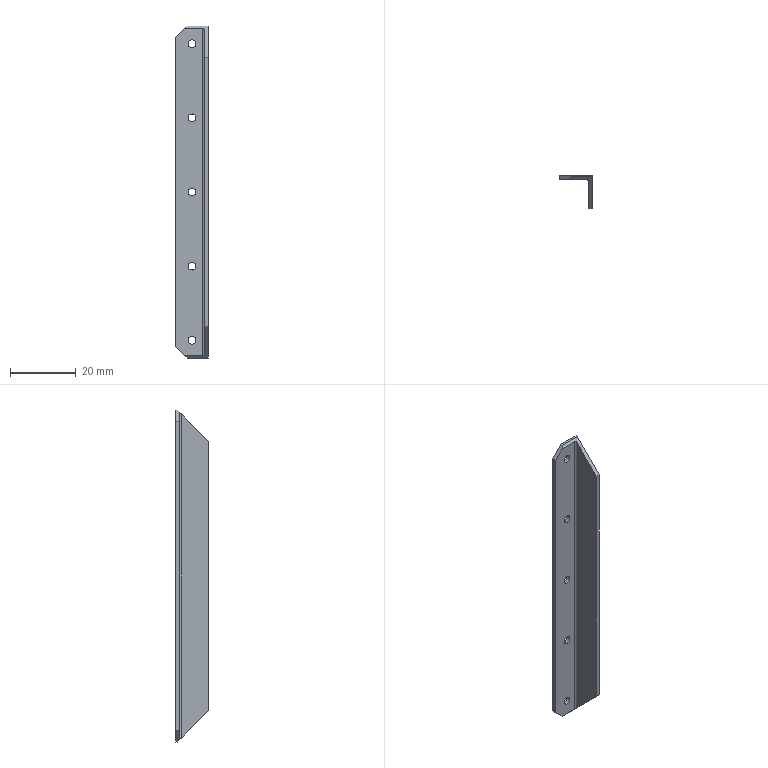Part | SolidWorks | features BaseBody 1 | 1 solid | 23 faces | box 10 x 10 x 100.8 mm | volume 2127 mm3 | plane 12 | cylinder 11 | commonest cylinder face diameters 2.4 x10 1 x1
STEP:
#1=CARTESIAN_POINT('',(-5.,-1.2,74.1));
#2=VERTEX_POINT('',#1);
#3=CARTESIAN_POINT('',(-5.,-1.2,71.7));
#4=VERTEX_POINT('',#3);
#5=CARTESIAN_POINT('',(-5.,-1.2,72.9));
#6=DIRECTION('',(0.,-1.,0.));
#7=DIRECTION('',(0.,0.,1.));
#8=AXIS2_PLACEMENT_3D('',#5,#6,#7);
#9=CIRCLE('',#8,1.2);
#10=EDGE_CURVE('',#2,#4,#9,.T.);
#11=ORIENTED_EDGE('',*,*,#10,.T.);
#12=CARTESIAN_POINT('',(-5.,0.,71.7));
#13=VERTEX_POINT('',#12);
#14=CARTESIAN_POINT('',(-5.,-1.2,71.7));
#15=DIRECTION('',(0.,1.,0.));
#16=VECTOR('',#15,1000.);
#17=LINE('',#14,#16);
#18=EDGE_CURVE('',#4,#13,#17,.T.);
#19=ORIENTED_EDGE('',*,*,#18,.T.);
#20=CARTESIAN_POINT('',(-5.,0.,74.1));
#21=VERTEX_POINT('',#20);
#22=CARTESIAN_POINT('',(-5.,0.,72.9));
#23=DIRECTION('',(0.,1.,0.));
#24=DIRECTION('',(0.,0.,1.));
#25=AXIS2_PLACEMENT_3D('',#22,#23,#24);
#26=CIRCLE('',#25,1.2);
#27=EDGE_CURVE('',#13,#21,#26,.T.);
#28=ORIENTED_EDGE('',*,*,#27,.T.);
#29=CARTESIAN_POINT('',(-5.,-1.2,74.1));
#30=DIRECTION('',(0.,1.,0.));
#31=VECTOR('',#30,1000.);
#32=LINE('',#29,#31);
#33=EDGE_CURVE('',#2,#21,#32,.T.);
#34=ORIENTED_EDGE('',*,*,#33,.F.);
#35=EDGE_LOOP('',(#11,#19,#28,#34));
#36=FACE_OUTER_BOUND('',#35,.T.);
#37=CARTESIAN_POINT('',(-5.,-1.2,72.9));
#38=DIRECTION('',(0.,1.,0.));
#39=DIRECTION('',(0.,0.,1.));
#40=AXIS2_PLACEMENT_3D('',#37,#38,#39);
#41=CYLINDRICAL_SURFACE('',#40,1.2);
#42=ADVANCED_FACE('',(#36),#41,.F.);
#43=CARTESIAN_POINT('',(-5.,-1.2,6.6));
#44=VERTEX_POINT('',#43);
#45=CARTESIAN_POINT('',(-5.,-1.2,4.2));
#46=VERTEX_POINT('',#45);
#47=CARTESIAN_POINT('',(-5.,-1.2,5.4));
#48=DIRECTION('',(0.,-1.,0.));
#49=DIRECTION('',(0.,0.,1.));
#50=AXIS2_PLACEMENT_3D('',#47,#48,#49);
#51=CIRCLE('',#50,1.2);
#52=EDGE_CURVE('',#44,#46,#51,.T.);
#53=ORIENTED_EDGE('',*,*,#52,.T.);
#54=CARTESIAN_POINT('',(-5.,0.,4.2));
#55=VERTEX_POINT('',#54);
#56=CARTESIAN_POINT('',(-5.,-1.2,4.2));
#57=DIRECTION('',(0.,1.,0.));
#58=VECTOR('',#57,1000.);
#59=LINE('',#56,#58);
#60=EDGE_CURVE('',#46,#55,#59,.T.);
#61=ORIENTED_EDGE('',*,*,#60,.T.);
#62=CARTESIAN_POINT('',(-5.,0.,6.6));
#63=VERTEX_POINT('',#62);
#64=CARTESIAN_POINT('',(-5.,0.,5.4));
#65=DIRECTION('',(0.,1.,0.));
#66=DIRECTION('',(0.,0.,1.));
#67=AXIS2_PLACEMENT_3D('',#64,#65,#66);
#68=CIRCLE('',#67,1.2);
#69=EDGE_CURVE('',#55,#63,#68,.T.);
#70=ORIENTED_EDGE('',*,*,#69,.T.);
#71=CARTESIAN_POINT('',(-5.,-1.2,6.6));
#72=DIRECTION('',(0.,1.,0.));
#73=VECTOR('',#72,1000.);
#74=LINE('',#71,#73);
#75=EDGE_CURVE('',#44,#63,#74,.T.);
#76=ORIENTED_EDGE('',*,*,#75,.F.);
#77=EDGE_LOOP('',(#53,#61,#70,#76));
#78=FACE_OUTER_BOUND('',#77,.T.);
#79=CARTESIAN_POINT('',(-5.,-1.2,5.4));
#80=DIRECTION('',(0.,1.,0.));
#81=DIRECTION('',(0.,0.,1.));
#82=AXIS2_PLACEMENT_3D('',#79,#80,#81);
#83=CYLINDRICAL_SURFACE('',#82,1.2);
#84=ADVANCED_FACE('',(#78),#83,.F.);
#85=CARTESIAN_POINT('',(-5.,-1.2,96.6));
#86=VERTEX_POINT('',#85);
#87=CARTESIAN_POINT('',(-5.,-1.2,94.2));
#88=VERTEX_POINT('',#87);
#89=CARTESIAN_POINT('',(-5.,-1.2,95.4));
#90=DIRECTION('',(0.,-1.,0.));
#91=DIRECTION('',(0.,0.,1.));
#92=AXIS2_PLACEMENT_3D('',#89,#90,#91);
#93=CIRCLE('',#92,1.2);
#94=EDGE_CURVE('',#86,#88,#93,.T.);
#95=ORIENTED_EDGE('',*,*,#94,.T.);
#96=CARTESIAN_POINT('',(-5.,0.,94.2));
#97=VERTEX_POINT('',#96);
#98=CARTESIAN_POINT('',(-5.,-1.2,94.2));
#99=DIRECTION('',(0.,1.,0.));
#100=VECTOR('',#99,1000.);
#101=LINE('',#98,#100);
#102=EDGE_CURVE('',#88,#97,#101,.T.);
#103=ORIENTED_EDGE('',*,*,#102,.T.);
#104=CARTESIAN_POINT('',(-5.,0.,96.6));
#105=VERTEX_POINT('',#104);
#106=CARTESIAN_POINT('',(-5.,0.,95.4));
#107=DIRECTION('',(0.,1.,0.));
#108=DIRECTION('',(0.,0.,1.));
#109=AXIS2_PLACEMENT_3D('',#106,#107,#108);
#110=CIRCLE('',#109,1.2);
#111=EDGE_CURVE('',#97,#105,#110,.T.);
#112=ORIENTED_EDGE('',*,*,#111,.T.);
#113=CARTESIAN_POINT('',(-5.,-1.2,96.6));
#114=DIRECTION('',(0.,1.,0.));
#115=VECTOR('',#114,1000.);
#116=LINE('',#113,#115);
#117=EDGE_CURVE('',#86,#105,#116,.T.);
#118=ORIENTED_EDGE('',*,*,#117,.F.);
#119=EDGE_LOOP('',(#95,#103,#112,#118));
#120=FACE_OUTER_BOUND('',#119,.T.);
#121=CARTESIAN_POINT('',(-5.,-1.2,95.4));
#122=DIRECTION('',(0.,1.,0.));
#123=DIRECTION('',(0.,0.,1.));
#124=AXIS2_PLACEMENT_3D('',#121,#122,#123);
#125=CYLINDRICAL_SURFACE('',#124,1.2);
#126=ADVANCED_FACE('',(#120),#125,.F.);
#127=CARTESIAN_POINT('',(-5.,-1.2,51.6));
#128=VERTEX_POINT('',#127);
#129=CARTESIAN_POINT('',(-5.,-1.2,49.2));
#130=VERTEX_POINT('',#129);
#131=CARTESIAN_POINT('',(-5.,-1.2,50.4));
#132=DIRECTION('',(0.,-1.,0.));
#133=DIRECTION('',(0.,0.,1.));
#134=AXIS2_PLACEMENT_3D('',#131,#132,#133);
#135=CIRCLE('',#134,1.2);
#136=EDGE_CURVE('',#128,#130,#135,.T.);
#137=ORIENTED_EDGE('',*,*,#136,.T.);
#138=CARTESIAN_POINT('',(-5.,0.,49.2));
#139=VERTEX_POINT('',#138);
#140=CARTESIAN_POINT('',(-5.,-1.2,49.2));
#141=DIRECTION('',(0.,1.,0.));
#142=VECTOR('',#141,1000.);
#143=LINE('',#140,#142);
#144=EDGE_CURVE('',#130,#139,#143,.T.);
#145=ORIENTED_EDGE('',*,*,#144,.T.);
#146=CARTESIAN_POINT('',(-5.,0.,51.6));
#147=VERTEX_POINT('',#146);
#148=CARTESIAN_POINT('',(-5.,0.,50.4));
#149=DIRECTION('',(0.,1.,0.));
#150=DIRECTION('',(0.,0.,1.));
#151=AXIS2_PLACEMENT_3D('',#148,#149,#150);
#152=CIRCLE('',#151,1.2);
#153=EDGE_CURVE('',#139,#147,#152,.T.);
#154=ORIENTED_EDGE('',*,*,#153,.T.);
#155=CARTESIAN_POINT('',(-5.,-1.2,51.6));
#156=DIRECTION('',(0.,1.,0.));
#157=VECTOR('',#156,1000.);
#158=LINE('',#155,#157);
#159=EDGE_CURVE('',#128,#147,#158,.T.);
#160=ORIENTED_EDGE('',*,*,#159,.F.);
#161=EDGE_LOOP('',(#137,#145,#154,#160));
#162=FACE_OUTER_BOUND('',#161,.T.);
#163=CARTESIAN_POINT('',(-5.,-1.2,50.4));
#164=DIRECTION('',(0.,1.,0.));
#165=DIRECTION('',(0.,0.,1.));
#166=AXIS2_PLACEMENT_3D('',#163,#164,#165);
#167=CYLINDRICAL_SURFACE('',#166,1.2);
#168=ADVANCED_FACE('',(#162),#167,.F.);
#169=CARTESIAN_POINT('',(-5.,-1.2,29.1));
#170=VERTEX_POINT('',#169);
#171=CARTESIAN_POINT('',(-5.,-1.2,26.7));
#172=VERTEX_POINT('',#171);
#173=CARTESIAN_POINT('',(-5.,-1.2,27.9));
#174=DIRECTION('',(0.,-1.,0.));
#175=DIRECTION('',(0.,0.,1.));
#176=AXIS2_PLACEMENT_3D('',#173,#174,#175);
#177=CIRCLE('',#176,1.2);
#178=EDGE_CURVE('',#170,#172,#177,.T.);
#179=ORIENTED_EDGE('',*,*,#178,.T.);
#180=CARTESIAN_POINT('',(-5.,0.,26.7));
#181=VERTEX_POINT('',#180);
#182=CARTESIAN_POINT('',(-5.,-1.2,26.7));
#183=DIRECTION('',(0.,1.,0.));
#184=VECTOR('',#183,1000.);
#185=LINE('',#182,#184);
#186=EDGE_CURVE('',#172,#181,#185,.T.);
#187=ORIENTED_EDGE('',*,*,#186,.T.);
#188=CARTESIAN_POINT('',(-5.,0.,29.1));
#189=VERTEX_POINT('',#188);
#190=CARTESIAN_POINT('',(-5.,0.,27.9));
#191=DIRECTION('',(0.,1.,0.));
#192=DIRECTION('',(0.,0.,1.));
#193=AXIS2_PLACEMENT_3D('',#190,#191,#192);
#194=CIRCLE('',#193,1.2);
#195=EDGE_CURVE('',#181,#189,#194,.T.);
#196=ORIENTED_EDGE('',*,*,#195,.T.);
#197=CARTESIAN_POINT('',(-5.,-1.2,29.1));
#198=DIRECTION('',(0.,1.,0.));
#199=VECTOR('',#198,1000.);
#200=LINE('',#197,#199);
#201=EDGE_CURVE('',#170,#189,#200,.T.);
#202=ORIENTED_EDGE('',*,*,#201,.F.);
#203=EDGE_LOOP('',(#179,#187,#196,#202));
#204=FACE_OUTER_BOUND('',#203,.T.);
#205=CARTESIAN_POINT('',(-5.,-1.2,27.9));
#206=DIRECTION('',(0.,1.,0.));
#207=DIRECTION('',(0.,0.,1.));
#208=AXIS2_PLACEMENT_3D('',#205,#206,#207);
#209=CYLINDRICAL_SURFACE('',#208,1.2);
#210=ADVANCED_FACE('',(#204),#209,.F.);
#211=ORIENTED_EDGE('',*,*,#18,.F.);
#212=CARTESIAN_POINT('',(-5.,-1.2,72.9));
#213=DIRECTION('',(0.,-1.,0.));
#214=DIRECTION('',(0.,0.,1.));
#215=AXIS2_PLACEMENT_3D('',#212,#213,#214);
#216=CIRCLE('',#215,1.2);
#217=EDGE_CURVE('',#4,#2,#216,.T.);
#218=ORIENTED_EDGE('',*,*,#217,.T.);
#219=ORIENTED_EDGE('',*,*,#33,.T.);
#220=CARTESIAN_POINT('',(-5.,0.,72.9));
#221=DIRECTION('',(0.,1.,0.));
#222=DIRECTION('',(0.,0.,1.));
#223=AXIS2_PLACEMENT_3D('',#220,#221,#222);
#224=CIRCLE('',#223,1.2);
#225=EDGE_CURVE('',#21,#13,#224,.T.);
#226=ORIENTED_EDGE('',*,*,#225,.T.);
#227=EDGE_LOOP('',(#211,#218,#219,#226));
#228=FACE_OUTER_BOUND('',#227,.T.);
#229=CARTESIAN_POINT('',(-5.,-1.2,72.9));
#230=DIRECTION('',(0.,1.,0.));
#231=DIRECTION('',(0.,0.,1.));
#232=AXIS2_PLACEMENT_3D('',#229,#230,#231);
#233=CYLINDRICAL_SURFACE('',#232,1.2);
#234=ADVANCED_FACE('',(#228),#233,.F.);
#235=CARTESIAN_POINT('',(-5.,0.,5.4));
#236=DIRECTION('',(0.,1.,0.));
#237=DIRECTION('',(0.,0.,1.));
#238=AXIS2_PLACEMENT_3D('',#235,#236,#237);
#239=CIRCLE('',#238,1.2);
#240=EDGE_CURVE('',#63,#55,#239,.T.);
#241=ORIENTED_EDGE('',*,*,#240,.F.);
#242=ORIENTED_EDGE('',*,*,#69,.F.);
#243=EDGE_LOOP('',(#241,#242));
#244=FACE_BOUND('',#243,.T.);
#245=CARTESIAN_POINT('',(-5.,0.,95.4));
#246=DIRECTION('',(0.,1.,0.));
#247=DIRECTION('',(0.,0.,1.));
#248=AXIS2_PLACEMENT_3D('',#245,#246,#247);
#249=CIRCLE('',#248,1.2);
#250=EDGE_CURVE('',#105,#97,#249,.T.);
#251=ORIENTED_EDGE('',*,*,#250,.F.);
#252=ORIENTED_EDGE('',*,*,#111,.F.);
#253=EDGE_LOOP('',(#251,#252));
#254=FACE_BOUND('',#253,.T.);
#255=CARTESIAN_POINT('',(-5.,0.,50.4));
#256=DIRECTION('',(0.,1.,0.));
#257=DIRECTION('',(0.,0.,1.));
#258=AXIS2_PLACEMENT_3D('',#255,#256,#257);
#259=CIRCLE('',#258,1.2);
#260=EDGE_CURVE('',#147,#139,#259,.T.);
#261=ORIENTED_EDGE('',*,*,#260,.F.);
#262=ORIENTED_EDGE('',*,*,#153,.F.);
#263=EDGE_LOOP('',(#261,#262));
#264=FACE_BOUND('',#263,.T.);
#265=CARTESIAN_POINT('',(-5.,0.,27.9));
#266=DIRECTION('',(0.,1.,0.));
#267=DIRECTION('',(0.,0.,1.));
#268=AXIS2_PLACEMENT_3D('',#265,#266,#267);
#269=CIRCLE('',#268,1.2);
#270=EDGE_CURVE('',#189,#181,#269,.T.);
#271=ORIENTED_EDGE('',*,*,#270,.F.);
#272=ORIENTED_EDGE('',*,*,#195,.F.);
#273=EDGE_LOOP('',(#271,#272));
#274=FACE_BOUND('',#273,.T.);
#275=ORIENTED_EDGE('',*,*,#225,.F.);
#276=ORIENTED_EDGE('',*,*,#27,.F.);
#277=EDGE_LOOP('',(#275,#276));
#278=FACE_BOUND('',#277,.T.);
#279=CARTESIAN_POINT('',(-6.5,0.,100.8));
#280=VERTEX_POINT('',#279);
#281=CARTESIAN_POINT('',(-10.,0.,97.3));
#282=VERTEX_POINT('',#281);
#283=CARTESIAN_POINT('',(-6.5,0.,100.8));
#284=DIRECTION('',(-0.7071,0.,-0.7071));
#285=VECTOR('',#284,1000.);
#286=LINE('',#283,#285);
#287=EDGE_CURVE('',#280,#282,#286,.T.);
#288=ORIENTED_EDGE('',*,*,#287,.F.);
#289=CARTESIAN_POINT('',(0.,0.,100.8));
#290=VERTEX_POINT('',#289);
#291=CARTESIAN_POINT('',(-5.,0.,100.8));
#292=DIRECTION('',(-1.,0.,0.));
#293=VECTOR('',#292,1000.);
#294=LINE('',#291,#293);
#295=EDGE_CURVE('',#290,#280,#294,.T.);
#296=ORIENTED_EDGE('',*,*,#295,.F.);
#297=CARTESIAN_POINT('',(0.,0.,0.));
#298=VERTEX_POINT('',#297);
#299=CARTESIAN_POINT('',(0.,0.,50.4));
#300=DIRECTION('',(0.,0.,1.));
#301=VECTOR('',#300,1000.);
#302=LINE('',#299,#301);
#303=EDGE_CURVE('',#298,#290,#302,.T.);
#304=ORIENTED_EDGE('',*,*,#303,.F.);
#305=CARTESIAN_POINT('',(-6.5,0.,0.));
#306=VERTEX_POINT('',#305);
#307=CARTESIAN_POINT('',(-5.,0.,0.));
#308=DIRECTION('',(1.,0.,0.));
#309=VECTOR('',#308,1000.);
#310=LINE('',#307,#309);
#311=EDGE_CURVE('',#306,#298,#310,.T.);
#312=ORIENTED_EDGE('',*,*,#311,.F.);
#313=CARTESIAN_POINT('',(-10.,0.,3.5));
#314=VERTEX_POINT('',#313);
#315=CARTESIAN_POINT('',(-6.5,0.,0.));
#316=DIRECTION('',(0.7071,0.,-0.7071));
#317=VECTOR('',#316,1000.);
#318=LINE('',#315,#317);
#319=EDGE_CURVE('',#314,#306,#318,.T.);
#320=ORIENTED_EDGE('',*,*,#319,.F.);
#321=CARTESIAN_POINT('',(-10.,0.,50.4));
#322=DIRECTION('',(0.,0.,-1.));
#323=VECTOR('',#322,1000.);
#324=LINE('',#321,#323);
#325=EDGE_CURVE('',#282,#314,#324,.T.);
#326=ORIENTED_EDGE('',*,*,#325,.F.);
#327=EDGE_LOOP('',(#288,#296,#304,#312,#320,#326));
#328=FACE_OUTER_BOUND('',#327,.T.);
#329=CARTESIAN_POINT('',(-10.,0.,0.));
#330=DIRECTION('',(0.,-1.,0.));
#331=DIRECTION('',(1.,0.,0.));
#332=AXIS2_PLACEMENT_3D('',#329,#330,#331);
#333=PLANE('',#332);
#334=ADVANCED_FACE('',(#244,#254,#264,#274,#278,#328),#333,.F.);
#335=ORIENTED_EDGE('',*,*,#52,.F.);
#336=CARTESIAN_POINT('',(-5.,-1.2,5.4));
#337=DIRECTION('',(0.,-1.,0.));
#338=DIRECTION('',(0.,0.,1.));
#339=AXIS2_PLACEMENT_3D('',#336,#337,#338);
#340=CIRCLE('',#339,1.2);
#341=EDGE_CURVE('',#46,#44,#340,.T.);
#342=ORIENTED_EDGE('',*,*,#341,.F.);
#343=EDGE_LOOP('',(#335,#342));
#344=FACE_BOUND('',#343,.T.);
#345=ORIENTED_EDGE('',*,*,#94,.F.);
#346=CARTESIAN_POINT('',(-5.,-1.2,95.4));
#347=DIRECTION('',(0.,-1.,0.));
#348=DIRECTION('',(0.,0.,1.));
#349=AXIS2_PLACEMENT_3D('',#346,#347,#348);
#350=CIRCLE('',#349,1.2);
#351=EDGE_CURVE('',#88,#86,#350,.T.);
#352=ORIENTED_EDGE('',*,*,#351,.F.);
#353=EDGE_LOOP('',(#345,#352));
#354=FACE_BOUND('',#353,.T.);
#355=ORIENTED_EDGE('',*,*,#136,.F.);
#356=CARTESIAN_POINT('',(-5.,-1.2,50.4));
#357=DIRECTION('',(0.,-1.,0.));
#358=DIRECTION('',(0.,0.,1.));
#359=AXIS2_PLACEMENT_3D('',#356,#357,#358);
#360=CIRCLE('',#359,1.2);
#361=EDGE_CURVE('',#130,#128,#360,.T.);
#362=ORIENTED_EDGE('',*,*,#361,.F.);
#363=EDGE_LOOP('',(#355,#362));
#364=FACE_BOUND('',#363,.T.);
#365=ORIENTED_EDGE('',*,*,#178,.F.);
#366=CARTESIAN_POINT('',(-5.,-1.2,27.9));
#367=DIRECTION('',(0.,-1.,0.));
#368=DIRECTION('',(0.,0.,1.));
#369=AXIS2_PLACEMENT_3D('',#366,#367,#368);
#370=CIRCLE('',#369,1.2);
#371=EDGE_CURVE('',#172,#170,#370,.T.);
#372=ORIENTED_EDGE('',*,*,#371,.F.);
#373=EDGE_LOOP('',(#365,#372));
#374=FACE_BOUND('',#373,.T.);
#375=ORIENTED_EDGE('',*,*,#10,.F.);
#376=ORIENTED_EDGE('',*,*,#217,.F.);
#377=EDGE_LOOP('',(#375,#376));
#378=FACE_BOUND('',#377,.T.);
#379=CARTESIAN_POINT('',(-1.7,-1.2,0.7));
#380=VERTEX_POINT('',#379);
#381=CARTESIAN_POINT('',(-7.2,-1.2,0.7));
#382=VERTEX_POINT('',#381);
#383=CARTESIAN_POINT('',(-5.85,-1.2,0.7));
#384=DIRECTION('',(-1.,0.,0.));
#385=VECTOR('',#384,1000.);
#386=LINE('',#383,#385);
#387=EDGE_CURVE('',#380,#382,#386,.T.);
#388=ORIENTED_EDGE('',*,*,#387,.F.);
#389=CARTESIAN_POINT('',(-1.7,-1.2,100.1));
#390=VERTEX_POINT('',#389);
#391=CARTESIAN_POINT('',(-1.7,-1.2,50.4));
#392=DIRECTION('',(0.,0.,-1.));
#393=VECTOR('',#392,1000.);
#394=LINE('',#391,#393);
#395=EDGE_CURVE('',#390,#380,#394,.T.);
#396=ORIENTED_EDGE('',*,*,#395,.F.);
#397=CARTESIAN_POINT('',(-7.2,-1.2,100.1));
#398=VERTEX_POINT('',#397);
#399=CARTESIAN_POINT('',(-5.85,-1.2,100.1));
#400=DIRECTION('',(1.,0.,0.));
#401=VECTOR('',#400,1000.);
#402=LINE('',#399,#401);
#403=EDGE_CURVE('',#398,#390,#402,.T.);
#404=ORIENTED_EDGE('',*,*,#403,.F.);
#405=CARTESIAN_POINT('',(-10.,-1.2,97.3));
#406=VERTEX_POINT('',#405);
#407=CARTESIAN_POINT('',(-6.5,-1.2,100.8));
#408=DIRECTION('',(0.7071,0.,0.7071));
#409=VECTOR('',#408,1000.);
#410=LINE('',#407,#409);
#411=EDGE_CURVE('',#406,#398,#410,.T.);
#412=ORIENTED_EDGE('',*,*,#411,.F.);
#413=CARTESIAN_POINT('',(-10.,-1.2,3.5));
#414=VERTEX_POINT('',#413);
#415=CARTESIAN_POINT('',(-10.,-1.2,50.4));
#416=DIRECTION('',(0.,0.,1.));
#417=VECTOR('',#416,1000.);
#418=LINE('',#415,#417);
#419=EDGE_CURVE('',#414,#406,#418,.T.);
#420=ORIENTED_EDGE('',*,*,#419,.F.);
#421=CARTESIAN_POINT('',(-6.5,-1.2,0.));
#422=DIRECTION('',(-0.7071,0.,0.7071));
#423=VECTOR('',#422,1000.);
#424=LINE('',#421,#423);
#425=EDGE_CURVE('',#382,#414,#424,.T.);
#426=ORIENTED_EDGE('',*,*,#425,.F.);
#427=EDGE_LOOP('',(#388,#396,#404,#412,#420,#426));
#428=FACE_OUTER_BOUND('',#427,.T.);
#429=CARTESIAN_POINT('',(-10.,-1.2,0.7));
#430=DIRECTION('',(0.,1.,0.));
#431=DIRECTION('',(0.,0.,1.));
#432=AXIS2_PLACEMENT_3D('',#429,#430,#431);
#433=PLANE('',#432);
#434=ADVANCED_FACE('',(#344,#354,#364,#374,#378,#428),#433,.F.);
#435=ORIENTED_EDGE('',*,*,#60,.F.);
#436=ORIENTED_EDGE('',*,*,#341,.T.);
#437=ORIENTED_EDGE('',*,*,#75,.T.);
#438=ORIENTED_EDGE('',*,*,#240,.T.);
#439=EDGE_LOOP('',(#435,#436,#437,#438));
#440=FACE_OUTER_BOUND('',#439,.T.);
#441=CARTESIAN_POINT('',(-5.,-1.2,5.4));
#442=DIRECTION('',(0.,1.,0.));
#443=DIRECTION('',(0.,0.,1.));
#444=AXIS2_PLACEMENT_3D('',#441,#442,#443);
#445=CYLINDRICAL_SURFACE('',#444,1.2);
#446=ADVANCED_FACE('',(#440),#445,.F.);
#447=ORIENTED_EDGE('',*,*,#102,.F.);
#448=ORIENTED_EDGE('',*,*,#351,.T.);
#449=ORIENTED_EDGE('',*,*,#117,.T.);
#450=ORIENTED_EDGE('',*,*,#250,.T.);
#451=EDGE_LOOP('',(#447,#448,#449,#450));
#452=FACE_OUTER_BOUND('',#451,.T.);
#453=CARTESIAN_POINT('',(-5.,-1.2,95.4));
#454=DIRECTION('',(0.,1.,0.));
#455=DIRECTION('',(0.,0.,1.));
#456=AXIS2_PLACEMENT_3D('',#453,#454,#455);
#457=CYLINDRICAL_SURFACE('',#456,1.2);
#458=ADVANCED_FACE('',(#452),#457,.F.);
#459=ORIENTED_EDGE('',*,*,#144,.F.);
#460=ORIENTED_EDGE('',*,*,#361,.T.);
#461=ORIENTED_EDGE('',*,*,#159,.T.);
#462=ORIENTED_EDGE('',*,*,#260,.T.);
#463=EDGE_LOOP('',(#459,#460,#461,#462));
#464=FACE_OUTER_BOUND('',#463,.T.);
#465=CARTESIAN_POINT('',(-5.,-1.2,50.4));
#466=DIRECTION('',(0.,1.,0.));
#467=DIRECTION('',(0.,0.,1.));
#468=AXIS2_PLACEMENT_3D('',#465,#466,#467);
#469=CYLINDRICAL_SURFACE('',#468,1.2);
#470=ADVANCED_FACE('',(#464),#469,.F.);
#471=ORIENTED_EDGE('',*,*,#186,.F.);
#472=ORIENTED_EDGE('',*,*,#371,.T.);
#473=ORIENTED_EDGE('',*,*,#201,.T.);
#474=ORIENTED_EDGE('',*,*,#270,.T.);
#475=EDGE_LOOP('',(#471,#472,#473,#474));
#476=FACE_OUTER_BOUND('',#475,.T.);
#477=CARTESIAN_POINT('',(-5.,-1.2,27.9));
#478=DIRECTION('',(0.,1.,0.));
#479=DIRECTION('',(0.,0.,1.));
#480=AXIS2_PLACEMENT_3D('',#477,#478,#479);
#481=CYLINDRICAL_SURFACE('',#480,1.2);
#482=ADVANCED_FACE('',(#476),#481,.F.);
#483=CARTESIAN_POINT('',(-10.,-0.6,97.3));
#484=DIRECTION('',(0.,-1.,0.));
#485=VECTOR('',#484,1000.);
#486=LINE('',#483,#485);
#487=EDGE_CURVE('',#282,#406,#486,.T.);
#488=ORIENTED_EDGE('',*,*,#487,.F.);
#489=ORIENTED_EDGE('',*,*,#325,.T.);
#490=CARTESIAN_POINT('',(-10.,-0.6,3.5));
#491=DIRECTION('',(0.,1.,0.));
#492=VECTOR('',#491,1000.);
#493=LINE('',#490,#492);
#494=EDGE_CURVE('',#414,#314,#493,.T.);
#495=ORIENTED_EDGE('',*,*,#494,.F.);
#496=ORIENTED_EDGE('',*,*,#419,.T.);
#497=EDGE_LOOP('',(#488,#489,#495,#496));
#498=FACE_OUTER_BOUND('',#497,.T.);
#499=CARTESIAN_POINT('',(-10.,-1.2,97.3));
#500=DIRECTION('',(1.,0.,0.));
#501=DIRECTION('',(0.,0.,-1.));
#502=AXIS2_PLACEMENT_3D('',#499,#500,#501);
#503=PLANE('',#502);
#504=ADVANCED_FACE('',(#498),#503,.F.);
#505=CARTESIAN_POINT('',(-6.5,-0.5,100.8));
#506=VERTEX_POINT('',#505);
#507=CARTESIAN_POINT('',(-6.5,-0.5,100.8));
#508=DIRECTION('',(-0.5774,-0.5774,-0.5774));
#509=VECTOR('',#508,1000.);
#510=LINE('',#507,#509);
#511=EDGE_CURVE('',#506,#398,#510,.T.);
#512=ORIENTED_EDGE('',*,*,#511,.F.);
#513=CARTESIAN_POINT('',(-6.5,-0.6,100.8));
#514=DIRECTION('',(0.,-1.,0.));
#515=VECTOR('',#514,1000.);
#516=LINE('',#513,#515);
#517=EDGE_CURVE('',#280,#506,#516,.T.);
#518=ORIENTED_EDGE('',*,*,#517,.F.);
#519=ORIENTED_EDGE('',*,*,#287,.T.);
#520=ORIENTED_EDGE('',*,*,#487,.T.);
#521=ORIENTED_EDGE('',*,*,#411,.T.);
#522=EDGE_LOOP('',(#512,#518,#519,#520,#521));
#523=FACE_OUTER_BOUND('',#522,.T.);
#524=CARTESIAN_POINT('',(-6.5,-1.2,100.8));
#525=DIRECTION('',(0.7071,0.,-0.7071));
#526=DIRECTION('',(-0.7071,0.,-0.7071));
#527=AXIS2_PLACEMENT_3D('',#524,#525,#526);
#528=PLANE('',#527);
#529=ADVANCED_FACE('',(#523),#528,.F.);
#530=CARTESIAN_POINT('',(0.,-0.5,100.8));
#531=VERTEX_POINT('',#530);
#532=CARTESIAN_POINT('',(-3.25,-0.5,100.8));
#533=DIRECTION('',(-1.,0.,0.));
#534=VECTOR('',#533,1000.);
#535=LINE('',#532,#534);
#536=EDGE_CURVE('',#531,#506,#535,.T.);
#537=ORIENTED_EDGE('',*,*,#536,.F.);
#538=CARTESIAN_POINT('',(0.,-0.25,100.8));
#539=DIRECTION('',(0.,-1.,0.));
#540=VECTOR('',#539,1000.);
#541=LINE('',#538,#540);
#542=EDGE_CURVE('',#290,#531,#541,.T.);
#543=ORIENTED_EDGE('',*,*,#542,.F.);
#544=ORIENTED_EDGE('',*,*,#295,.T.);
#545=ORIENTED_EDGE('',*,*,#517,.T.);
#546=EDGE_LOOP('',(#537,#543,#544,#545));
#547=FACE_OUTER_BOUND('',#546,.T.);
#548=CARTESIAN_POINT('',(0.,-0.5,100.8));
#549=DIRECTION('',(0.,0.,-1.));
#550=DIRECTION('',(-1.,0.,0.));
#551=AXIS2_PLACEMENT_3D('',#548,#549,#550);
#552=PLANE('',#551);
#553=ADVANCED_FACE('',(#547),#552,.F.);
#554=CARTESIAN_POINT('',(0.,-0.5,0.));
#555=VERTEX_POINT('',#554);
#556=CARTESIAN_POINT('',(0.,-10.,9.5));
#557=VERTEX_POINT('',#556);
#558=CARTESIAN_POINT('',(0.,-10.,9.5));
#559=DIRECTION('',(0.,-0.7071,0.7071));
#560=VECTOR('',#559,1000.);
#561=LINE('',#558,#560);
#562=EDGE_CURVE('',#555,#557,#561,.T.);
#563=ORIENTED_EDGE('',*,*,#562,.F.);
#564=CARTESIAN_POINT('',(0.,-5.,0.));
#565=DIRECTION('',(0.,-1.,0.));
#566=VECTOR('',#565,1000.);
#567=LINE('',#564,#566);
#568=EDGE_CURVE('',#298,#555,#567,.T.);
#569=ORIENTED_EDGE('',*,*,#568,.F.);
#570=ORIENTED_EDGE('',*,*,#303,.T.);
#571=ORIENTED_EDGE('',*,*,#542,.T.);
#572=CARTESIAN_POINT('',(0.,-10.,91.3));
#573=VERTEX_POINT('',#572);
#574=CARTESIAN_POINT('',(0.,-10.,91.3));
#575=DIRECTION('',(0.,0.7071,0.7071));
#576=VECTOR('',#575,1000.);
#577=LINE('',#574,#576);
#578=EDGE_CURVE('',#573,#531,#577,.T.);
#579=ORIENTED_EDGE('',*,*,#578,.F.);
#580=CARTESIAN_POINT('',(0.,-10.,50.4));
#581=DIRECTION('',(0.,0.,1.));
#582=VECTOR('',#581,1000.);
#583=LINE('',#580,#582);
#584=EDGE_CURVE('',#557,#573,#583,.T.);
#585=ORIENTED_EDGE('',*,*,#584,.F.);
#586=EDGE_LOOP('',(#563,#569,#570,#571,#579,#585));
#587=FACE_OUTER_BOUND('',#586,.T.);
#588=CARTESIAN_POINT('',(0.,0.,0.));
#589=DIRECTION('',(-1.,0.,0.));
#590=DIRECTION('',(0.,-1.,0.));
#591=AXIS2_PLACEMENT_3D('',#588,#589,#590);
#592=PLANE('',#591);
#593=ADVANCED_FACE('',(#587),#592,.F.);
#594=CARTESIAN_POINT('',(-6.5,-0.5,0.));
#595=VERTEX_POINT('',#594);
#596=CARTESIAN_POINT('',(-6.5,-0.25,0.));
#597=DIRECTION('',(0.,1.,0.));
#598=VECTOR('',#597,1000.);
#599=LINE('',#596,#598);
#600=EDGE_CURVE('',#595,#306,#599,.T.);
#601=ORIENTED_EDGE('',*,*,#600,.T.);
#602=ORIENTED_EDGE('',*,*,#311,.T.);
#603=ORIENTED_EDGE('',*,*,#568,.T.);
#604=CARTESIAN_POINT('',(-3.25,-0.5,0.));
#605=DIRECTION('',(-1.,0.,0.));
#606=VECTOR('',#605,1000.);
#607=LINE('',#604,#606);
#608=EDGE_CURVE('',#555,#595,#607,.T.);
#609=ORIENTED_EDGE('',*,*,#608,.T.);
#610=EDGE_LOOP('',(#601,#602,#603,#609));
#611=FACE_OUTER_BOUND('',#610,.T.);
#612=CARTESIAN_POINT('',(0.,-0.5,0.));
#613=DIRECTION('',(0.,0.,-1.));
#614=DIRECTION('',(-1.,0.,0.));
#615=AXIS2_PLACEMENT_3D('',#612,#613,#614);
#616=PLANE('',#615);
#617=ADVANCED_FACE('',(#611),#616,.T.);
#618=ORIENTED_EDGE('',*,*,#494,.T.);
#619=ORIENTED_EDGE('',*,*,#319,.T.);
#620=ORIENTED_EDGE('',*,*,#600,.F.);
#621=CARTESIAN_POINT('',(-6.5,-0.5,0.));
#622=DIRECTION('',(-0.5774,-0.5774,0.5774));
#623=VECTOR('',#622,1000.);
#624=LINE('',#621,#623);
#625=EDGE_CURVE('',#595,#382,#624,.T.);
#626=ORIENTED_EDGE('',*,*,#625,.T.);
#627=ORIENTED_EDGE('',*,*,#425,.T.);
#628=EDGE_LOOP('',(#618,#619,#620,#626,#627));
#629=FACE_OUTER_BOUND('',#628,.T.);
#630=CARTESIAN_POINT('',(-6.5,-1.2,0.));
#631=DIRECTION('',(-0.7071,0.,-0.7071));
#632=DIRECTION('',(-0.7071,0.,0.7071));
#633=AXIS2_PLACEMENT_3D('',#630,#631,#632);
#634=PLANE('',#633);
#635=ADVANCED_FACE('',(#629),#634,.T.);
#636=CARTESIAN_POINT('',(-1.2,-1.7,1.2));
#637=VERTEX_POINT('',#636);
#638=CARTESIAN_POINT('',(-1.2,-1.7,1.2));
#639=CARTESIAN_POINT('',(-1.2,-1.407,0.9071));
#640=CARTESIAN_POINT('',(-1.407,-1.2,0.7));
#641=CARTESIAN_POINT('',(-1.7,-1.2,0.7));
#642=(BOUNDED_CURVE()B_SPLINE_CURVE(3,(#638,#639,#640,#641),.UNSPECIFIED.,.F.,.F.)B_SPLINE_CURVE_WITH_KNOTS((4,4),(4.712,6.283),.UNSPECIFIED.)CURVE()GEOMETRIC_REPRESENTATION_ITEM()RATIONAL_B_SPLINE_CURVE((1.,0.8047,0.8047,1.))REPRESENTATION_ITEM(''));
#643=EDGE_CURVE('',#637,#380,#642,.T.);
#644=ORIENTED_EDGE('',*,*,#643,.T.);
#645=ORIENTED_EDGE('',*,*,#387,.T.);
#646=ORIENTED_EDGE('',*,*,#625,.F.);
#647=ORIENTED_EDGE('',*,*,#608,.F.);
#648=ORIENTED_EDGE('',*,*,#562,.T.);
#649=CARTESIAN_POINT('',(-1.2,-10.,9.5));
#650=VERTEX_POINT('',#649);
#651=CARTESIAN_POINT('',(-3.622,-10.,9.5));
#652=DIRECTION('',(-1.,0.,0.));
#653=VECTOR('',#652,1000.);
#654=LINE('',#651,#653);
#655=EDGE_CURVE('',#557,#650,#654,.T.);
#656=ORIENTED_EDGE('',*,*,#655,.T.);
#657=CARTESIAN_POINT('',(-1.2,-5.25,4.75));
#658=DIRECTION('',(0.,0.7071,-0.7071));
#659=VECTOR('',#658,1000.);
#660=LINE('',#657,#659);
#661=EDGE_CURVE('',#650,#637,#660,.T.);
#662=ORIENTED_EDGE('',*,*,#661,.T.);
#663=EDGE_LOOP('',(#644,#645,#646,#647,#648,#656,#662));
#664=FACE_OUTER_BOUND('',#663,.T.);
#665=CARTESIAN_POINT('',(-7.243,-10.,9.5));
#666=DIRECTION('',(0.,-0.7071,-0.7071));
#667=DIRECTION('',(0.,0.7071,-0.7071));
#668=AXIS2_PLACEMENT_3D('',#665,#666,#667);
#669=PLANE('',#668);
#670=ADVANCED_FACE('',(#664),#669,.T.);
#671=CARTESIAN_POINT('',(-1.2,-1.7,99.6));
#672=VERTEX_POINT('',#671);
#673=CARTESIAN_POINT('',(-1.2,-1.7,50.4));
#674=DIRECTION('',(0.,0.,1.));
#675=VECTOR('',#674,1000.);
#676=LINE('',#673,#675);
#677=EDGE_CURVE('',#637,#672,#676,.T.);
#678=ORIENTED_EDGE('',*,*,#677,.T.);
#679=CARTESIAN_POINT('',(-1.2,-1.7,99.6));
#680=CARTESIAN_POINT('',(-1.2,-1.407,99.893));
#681=CARTESIAN_POINT('',(-1.407,-1.2,100.1));
#682=CARTESIAN_POINT('',(-1.7,-1.2,100.1));
#683=(BOUNDED_CURVE()B_SPLINE_CURVE(3,(#679,#680,#681,#682),.UNSPECIFIED.,.F.,.F.)B_SPLINE_CURVE_WITH_KNOTS((4,4),(1.571,3.142),.UNSPECIFIED.)CURVE()GEOMETRIC_REPRESENTATION_ITEM()RATIONAL_B_SPLINE_CURVE((1.,0.8047,0.8047,1.))REPRESENTATION_ITEM(''));
#684=EDGE_CURVE('',#672,#390,#683,.T.);
#685=ORIENTED_EDGE('',*,*,#684,.T.);
#686=ORIENTED_EDGE('',*,*,#395,.T.);
#687=ORIENTED_EDGE('',*,*,#643,.F.);
#688=EDGE_LOOP('',(#678,#685,#686,#687));
#689=FACE_OUTER_BOUND('',#688,.T.);
#690=CARTESIAN_POINT('',(-1.7,-1.7,100.696));
#691=DIRECTION('',(0.,0.,-1.));
#692=DIRECTION('',(-1.,0.,0.));
#693=AXIS2_PLACEMENT_3D('',#690,#691,#692);
#694=CYLINDRICAL_SURFACE('',#693,0.5);
#695=ADVANCED_FACE('',(#689),#694,.F.);
#696=CARTESIAN_POINT('',(-1.2,-10.,91.3));
#697=VERTEX_POINT('',#696);
#698=CARTESIAN_POINT('',(-3.622,-10.,91.3));
#699=DIRECTION('',(-1.,0.,0.));
#700=VECTOR('',#699,1000.);
#701=LINE('',#698,#700);
#702=EDGE_CURVE('',#573,#697,#701,.T.);
#703=ORIENTED_EDGE('',*,*,#702,.F.);
#704=ORIENTED_EDGE('',*,*,#578,.T.);
#705=ORIENTED_EDGE('',*,*,#536,.T.);
#706=ORIENTED_EDGE('',*,*,#511,.T.);
#707=ORIENTED_EDGE('',*,*,#403,.T.);
#708=ORIENTED_EDGE('',*,*,#684,.F.);
#709=CARTESIAN_POINT('',(-1.2,-5.25,96.05));
#710=DIRECTION('',(0.,0.7071,0.7071));
#711=VECTOR('',#710,1000.);
#712=LINE('',#709,#711);
#713=EDGE_CURVE('',#697,#672,#712,.T.);
#714=ORIENTED_EDGE('',*,*,#713,.F.);
#715=EDGE_LOOP('',(#703,#704,#705,#706,#707,#708,#714));
#716=FACE_OUTER_BOUND('',#715,.T.);
#717=CARTESIAN_POINT('',(-7.243,-10.,91.3));
#718=DIRECTION('',(0.,0.7071,-0.7071));
#719=DIRECTION('',(0.,0.7071,0.7071));
#720=AXIS2_PLACEMENT_3D('',#717,#718,#719);
#721=PLANE('',#720);
#722=ADVANCED_FACE('',(#716),#721,.F.);
#723=ORIENTED_EDGE('',*,*,#655,.F.);
#724=ORIENTED_EDGE('',*,*,#584,.T.);
#725=ORIENTED_EDGE('',*,*,#702,.T.);
#726=CARTESIAN_POINT('',(-1.2,-10.,50.4));
#727=DIRECTION('',(0.,0.,1.));
#728=VECTOR('',#727,1000.);
#729=LINE('',#726,#728);
#730=EDGE_CURVE('',#650,#697,#729,.T.);
#731=ORIENTED_EDGE('',*,*,#730,.F.);
#732=EDGE_LOOP('',(#723,#724,#725,#731));
#733=FACE_OUTER_BOUND('',#732,.T.);
#734=CARTESIAN_POINT('',(-1.2,-10.,9.5));
#735=DIRECTION('',(0.,1.,0.));
#736=DIRECTION('',(0.,0.,1.));
#737=AXIS2_PLACEMENT_3D('',#734,#735,#736);
#738=PLANE('',#737);
#739=ADVANCED_FACE('',(#733),#738,.F.);
#740=ORIENTED_EDGE('',*,*,#661,.F.);
#741=ORIENTED_EDGE('',*,*,#730,.T.);
#742=ORIENTED_EDGE('',*,*,#713,.T.);
#743=ORIENTED_EDGE('',*,*,#677,.F.);
#744=EDGE_LOOP('',(#740,#741,#742,#743));
#745=FACE_OUTER_BOUND('',#744,.T.);
#746=CARTESIAN_POINT('',(-1.2,-10.,100.19));
#747=DIRECTION('',(1.,0.,0.));
#748=DIRECTION('',(0.,0.,-1.));
#749=AXIS2_PLACEMENT_3D('',#746,#747,#748);
#750=PLANE('',#749);
#751=ADVANCED_FACE('',(#745),#750,.F.);
#752=CLOSED_SHELL('',(#42,#84,#126,#168,#210,#234,#334,#434,#446,#458,#470,#482,#504,#529,#553,#593,#617,#635,#670,#695,#722,#739,#751));
#753=MANIFOLD_SOLID_BREP('',#752);
#754=CARTESIAN_POINT('',(0.,0.,0.));
#755=DIRECTION('',(0.,0.,1.));
#756=DIRECTION('',(1.,0.,0.));
#757=AXIS2_PLACEMENT_3D('',#754,#755,#756);
#758=(LENGTH_UNIT()NAMED_UNIT(*)SI_UNIT(.MILLI.,.METRE.));
#759=UNCERTAINTY_MEASURE_WITH_UNIT(LENGTH_MEASURE(0.00001),#758,'','');
#760=(NAMED_UNIT(*)PLANE_ANGLE_UNIT()SI_UNIT($,.RADIAN.));
#761=(NAMED_UNIT(*)SI_UNIT($,.STERADIAN.)SOLID_ANGLE_UNIT());
#762=(GEOMETRIC_REPRESENTATION_CONTEXT(3)GLOBAL_UNCERTAINTY_ASSIGNED_CONTEXT((#759))GLOBAL_UNIT_ASSIGNED_CONTEXT((#758,#760,#761))REPRESENTATION_CONTEXT('',''));
#763=ADVANCED_BREP_SHAPE_REPRESENTATION('',(#753,#757),#762);